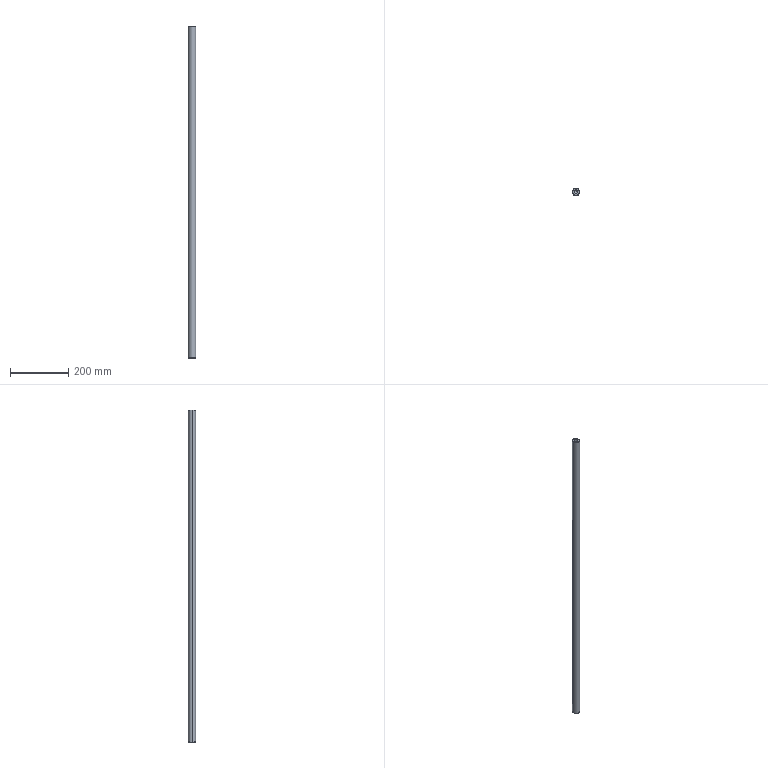Part | SolidWorks | features BaseBody 1 | 1 solid | 16 faces | box 25 x 25 x 1142 mm | volume 551182 mm3 | cone 8 | cylinder 6 | plane 2 | commonest cylinder face diameters 12 x4 25 x2
STEP:
#1=CARTESIAN_POINT('',(-11.5,0.,-571.));
#2=VERTEX_POINT('',#1);
#3=CARTESIAN_POINT('',(-12.5,0.,-570.));
#4=VERTEX_POINT('',#3);
#5=CARTESIAN_POINT('',(-12.5,0.,-570.));
#6=DIRECTION('',(-0.7071,0.,0.7071));
#7=VECTOR('',#6,1000.);
#8=LINE('',#5,#7);
#9=EDGE_CURVE('',#2,#4,#8,.T.);
#10=ORIENTED_EDGE('',*,*,#9,.F.);
#11=CARTESIAN_POINT('',(11.5,0.,-571.));
#12=VERTEX_POINT('',#11);
#13=CARTESIAN_POINT('',(0.,0.,-571.));
#14=DIRECTION('',(0.,0.,-1.));
#15=DIRECTION('',(1.,0.,0.));
#16=AXIS2_PLACEMENT_3D('',#13,#14,#15);
#17=CIRCLE('',#16,11.5);
#18=EDGE_CURVE('',#12,#2,#17,.T.);
#19=ORIENTED_EDGE('',*,*,#18,.F.);
#20=CARTESIAN_POINT('',(12.5,0.,-570.));
#21=VERTEX_POINT('',#20);
#22=CARTESIAN_POINT('',(12.5,0.,-570.));
#23=DIRECTION('',(0.7071,0.,0.7071));
#24=VECTOR('',#23,1000.);
#25=LINE('',#22,#24);
#26=EDGE_CURVE('',#12,#21,#25,.T.);
#27=ORIENTED_EDGE('',*,*,#26,.T.);
#28=CARTESIAN_POINT('',(0.,0.,-570.));
#29=DIRECTION('',(0.,0.,1.));
#30=DIRECTION('',(1.,0.,0.));
#31=AXIS2_PLACEMENT_3D('',#28,#29,#30);
#32=CIRCLE('',#31,12.5);
#33=EDGE_CURVE('',#4,#21,#32,.T.);
#34=ORIENTED_EDGE('',*,*,#33,.F.);
#35=EDGE_LOOP('',(#10,#19,#27,#34));
#36=FACE_OUTER_BOUND('',#35,.T.);
#37=CARTESIAN_POINT('',(0.,0.,-570.));
#38=DIRECTION('',(0.,0.,1.));
#39=DIRECTION('',(1.,0.,0.));
#40=AXIS2_PLACEMENT_3D('',#37,#38,#39);
#41=CONICAL_SURFACE('',#40,12.5,0.7854);
#42=ADVANCED_FACE('',(#36),#41,.T.);
#43=CARTESIAN_POINT('',(11.5,0.,571.));
#44=VERTEX_POINT('',#43);
#45=CARTESIAN_POINT('',(12.5,0.,570.));
#46=VERTEX_POINT('',#45);
#47=CARTESIAN_POINT('',(11.5,0.,571.));
#48=DIRECTION('',(0.7071,0.,-0.7071));
#49=VECTOR('',#48,1000.);
#50=LINE('',#47,#49);
#51=EDGE_CURVE('',#44,#46,#50,.T.);
#52=ORIENTED_EDGE('',*,*,#51,.F.);
#53=CARTESIAN_POINT('',(-11.5,0.,571.));
#54=VERTEX_POINT('',#53);
#55=CARTESIAN_POINT('',(0.,0.,571.));
#56=DIRECTION('',(0.,0.,1.));
#57=DIRECTION('',(1.,0.,0.));
#58=AXIS2_PLACEMENT_3D('',#55,#56,#57);
#59=CIRCLE('',#58,11.5);
#60=EDGE_CURVE('',#54,#44,#59,.T.);
#61=ORIENTED_EDGE('',*,*,#60,.F.);
#62=CARTESIAN_POINT('',(-12.5,0.,570.));
#63=VERTEX_POINT('',#62);
#64=CARTESIAN_POINT('',(-11.5,0.,571.));
#65=DIRECTION('',(-0.7071,0.,-0.7071));
#66=VECTOR('',#65,1000.);
#67=LINE('',#64,#66);
#68=EDGE_CURVE('',#54,#63,#67,.T.);
#69=ORIENTED_EDGE('',*,*,#68,.T.);
#70=CARTESIAN_POINT('',(0.,0.,570.));
#71=DIRECTION('',(0.,0.,-1.));
#72=DIRECTION('',(1.,0.,0.));
#73=AXIS2_PLACEMENT_3D('',#70,#71,#72);
#74=CIRCLE('',#73,12.5);
#75=EDGE_CURVE('',#46,#63,#74,.T.);
#76=ORIENTED_EDGE('',*,*,#75,.F.);
#77=EDGE_LOOP('',(#52,#61,#69,#76));
#78=FACE_OUTER_BOUND('',#77,.T.);
#79=CARTESIAN_POINT('',(0.,0.,571.));
#80=DIRECTION('',(0.,0.,-1.));
#81=DIRECTION('',(-1.,0.,0.));
#82=AXIS2_PLACEMENT_3D('',#79,#80,#81);
#83=CONICAL_SURFACE('',#82,11.5,0.7854);
#84=ADVANCED_FACE('',(#78),#83,.T.);
#85=CARTESIAN_POINT('',(6.,0.,-531.));
#86=VERTEX_POINT('',#85);
#87=CARTESIAN_POINT('',(6.,0.,-571.));
#88=VERTEX_POINT('',#87);
#89=CARTESIAN_POINT('',(6.,0.,-571.));
#90=DIRECTION('',(0.,0.,-1.));
#91=VECTOR('',#90,1000.);
#92=LINE('',#89,#91);
#93=EDGE_CURVE('',#86,#88,#92,.T.);
#94=ORIENTED_EDGE('',*,*,#93,.F.);
#95=CARTESIAN_POINT('',(-6.,0.,-531.));
#96=VERTEX_POINT('',#95);
#97=CARTESIAN_POINT('',(0.,0.,-531.));
#98=DIRECTION('',(0.,0.,-1.));
#99=DIRECTION('',(-1.,0.,0.));
#100=AXIS2_PLACEMENT_3D('',#97,#98,#99);
#101=CIRCLE('',#100,6.);
#102=EDGE_CURVE('',#96,#86,#101,.T.);
#103=ORIENTED_EDGE('',*,*,#102,.F.);
#104=CARTESIAN_POINT('',(-6.,0.,-571.));
#105=VERTEX_POINT('',#104);
#106=CARTESIAN_POINT('',(-6.,0.,-571.));
#107=DIRECTION('',(0.,0.,-1.));
#108=VECTOR('',#107,1000.);
#109=LINE('',#106,#108);
#110=EDGE_CURVE('',#96,#105,#109,.T.);
#111=ORIENTED_EDGE('',*,*,#110,.T.);
#112=CARTESIAN_POINT('',(0.,0.,-571.));
#113=DIRECTION('',(0.,0.,-1.));
#114=DIRECTION('',(-1.,0.,0.));
#115=AXIS2_PLACEMENT_3D('',#112,#113,#114);
#116=CIRCLE('',#115,6.);
#117=EDGE_CURVE('',#105,#88,#116,.T.);
#118=ORIENTED_EDGE('',*,*,#117,.T.);
#119=EDGE_LOOP('',(#94,#103,#111,#118));
#120=FACE_OUTER_BOUND('',#119,.T.);
#121=CARTESIAN_POINT('',(0.,0.,-571.));
#122=DIRECTION('',(0.,0.,-1.));
#123=DIRECTION('',(-1.,0.,0.));
#124=AXIS2_PLACEMENT_3D('',#121,#122,#123);
#125=CYLINDRICAL_SURFACE('',#124,6.);
#126=ADVANCED_FACE('',(#120),#125,.F.);
#127=CARTESIAN_POINT('',(0.,0.,-527.395));
#128=VERTEX_POINT('',#127);
#129=CARTESIAN_POINT('',(6.,0.,-531.));
#130=DIRECTION('',(0.8572,0.,-0.515));
#131=VECTOR('',#130,1000.);
#132=LINE('',#129,#131);
#133=EDGE_CURVE('',#128,#86,#132,.T.);
#134=ORIENTED_EDGE('',*,*,#133,.F.);
#135=CARTESIAN_POINT('',(-6.,0.,-531.));
#136=DIRECTION('',(-0.8572,0.,-0.515));
#137=VECTOR('',#136,1000.);
#138=LINE('',#135,#137);
#139=EDGE_CURVE('',#128,#96,#138,.T.);
#140=ORIENTED_EDGE('',*,*,#139,.T.);
#141=ORIENTED_EDGE('',*,*,#102,.T.);
#142=EDGE_LOOP('',(#134,#140,#141));
#143=FACE_OUTER_BOUND('',#142,.T.);
#144=CARTESIAN_POINT('',(0.,0.,-531.));
#145=DIRECTION('',(0.,0.,-1.));
#146=DIRECTION('',(-1.,0.,0.));
#147=AXIS2_PLACEMENT_3D('',#144,#145,#146);
#148=CONICAL_SURFACE('',#147,6.,1.03);
#149=ADVANCED_FACE('',(#143),#148,.F.);
#150=CARTESIAN_POINT('',(-6.,0.,531.));
#151=VERTEX_POINT('',#150);
#152=CARTESIAN_POINT('',(-6.,0.,571.));
#153=VERTEX_POINT('',#152);
#154=CARTESIAN_POINT('',(-6.,0.,571.));
#155=DIRECTION('',(0.,0.,1.));
#156=VECTOR('',#155,1000.);
#157=LINE('',#154,#156);
#158=EDGE_CURVE('',#151,#153,#157,.T.);
#159=ORIENTED_EDGE('',*,*,#158,.F.);
#160=CARTESIAN_POINT('',(6.,0.,531.));
#161=VERTEX_POINT('',#160);
#162=CARTESIAN_POINT('',(0.,0.,531.));
#163=DIRECTION('',(0.,0.,1.));
#164=DIRECTION('',(1.,0.,0.));
#165=AXIS2_PLACEMENT_3D('',#162,#163,#164);
#166=CIRCLE('',#165,6.);
#167=EDGE_CURVE('',#161,#151,#166,.T.);
#168=ORIENTED_EDGE('',*,*,#167,.F.);
#169=CARTESIAN_POINT('',(6.,0.,571.));
#170=VERTEX_POINT('',#169);
#171=CARTESIAN_POINT('',(6.,0.,571.));
#172=DIRECTION('',(0.,0.,1.));
#173=VECTOR('',#172,1000.);
#174=LINE('',#171,#173);
#175=EDGE_CURVE('',#161,#170,#174,.T.);
#176=ORIENTED_EDGE('',*,*,#175,.T.);
#177=CARTESIAN_POINT('',(0.,0.,571.));
#178=DIRECTION('',(0.,0.,1.));
#179=DIRECTION('',(1.,0.,0.));
#180=AXIS2_PLACEMENT_3D('',#177,#178,#179);
#181=CIRCLE('',#180,6.);
#182=EDGE_CURVE('',#170,#153,#181,.T.);
#183=ORIENTED_EDGE('',*,*,#182,.T.);
#184=EDGE_LOOP('',(#159,#168,#176,#183));
#185=FACE_OUTER_BOUND('',#184,.T.);
#186=CARTESIAN_POINT('',(0.,0.,571.));
#187=DIRECTION('',(0.,0.,1.));
#188=DIRECTION('',(1.,0.,0.));
#189=AXIS2_PLACEMENT_3D('',#186,#187,#188);
#190=CYLINDRICAL_SURFACE('',#189,6.);
#191=ADVANCED_FACE('',(#185),#190,.F.);
#192=CARTESIAN_POINT('',(0.,0.,527.395));
#193=VERTEX_POINT('',#192);
#194=CARTESIAN_POINT('',(-6.,0.,531.));
#195=DIRECTION('',(-0.8572,0.,0.515));
#196=VECTOR('',#195,1000.);
#197=LINE('',#194,#196);
#198=EDGE_CURVE('',#193,#151,#197,.T.);
#199=ORIENTED_EDGE('',*,*,#198,.F.);
#200=CARTESIAN_POINT('',(6.,0.,531.));
#201=DIRECTION('',(0.8572,0.,0.515));
#202=VECTOR('',#201,1000.);
#203=LINE('',#200,#202);
#204=EDGE_CURVE('',#193,#161,#203,.T.);
#205=ORIENTED_EDGE('',*,*,#204,.T.);
#206=ORIENTED_EDGE('',*,*,#167,.T.);
#207=EDGE_LOOP('',(#199,#205,#206));
#208=FACE_OUTER_BOUND('',#207,.T.);
#209=CARTESIAN_POINT('',(0.,0.,531.));
#210=DIRECTION('',(0.,0.,1.));
#211=DIRECTION('',(1.,0.,0.));
#212=AXIS2_PLACEMENT_3D('',#209,#210,#211);
#213=CONICAL_SURFACE('',#212,6.,1.03);
#214=ADVANCED_FACE('',(#208),#213,.F.);
#215=ORIENTED_EDGE('',*,*,#117,.F.);
#216=CARTESIAN_POINT('',(0.,0.,-571.));
#217=DIRECTION('',(0.,0.,-1.));
#218=DIRECTION('',(-1.,0.,0.));
#219=AXIS2_PLACEMENT_3D('',#216,#217,#218);
#220=CIRCLE('',#219,6.);
#221=EDGE_CURVE('',#88,#105,#220,.T.);
#222=ORIENTED_EDGE('',*,*,#221,.F.);
#223=EDGE_LOOP('',(#215,#222));
#224=FACE_BOUND('',#223,.T.);
#225=ORIENTED_EDGE('',*,*,#18,.T.);
#226=CARTESIAN_POINT('',(0.,0.,-571.));
#227=DIRECTION('',(0.,0.,-1.));
#228=DIRECTION('',(1.,0.,0.));
#229=AXIS2_PLACEMENT_3D('',#226,#227,#228);
#230=CIRCLE('',#229,11.5);
#231=EDGE_CURVE('',#2,#12,#230,.T.);
#232=ORIENTED_EDGE('',*,*,#231,.T.);
#233=EDGE_LOOP('',(#225,#232));
#234=FACE_OUTER_BOUND('',#233,.T.);
#235=CARTESIAN_POINT('',(0.,0.,-571.));
#236=DIRECTION('',(0.,0.,1.));
#237=DIRECTION('',(1.,0.,0.));
#238=AXIS2_PLACEMENT_3D('',#235,#236,#237);
#239=PLANE('',#238);
#240=ADVANCED_FACE('',(#224,#234),#239,.F.);
#241=ORIENTED_EDGE('',*,*,#182,.F.);
#242=CARTESIAN_POINT('',(0.,0.,571.));
#243=DIRECTION('',(0.,0.,1.));
#244=DIRECTION('',(1.,0.,0.));
#245=AXIS2_PLACEMENT_3D('',#242,#243,#244);
#246=CIRCLE('',#245,6.);
#247=EDGE_CURVE('',#153,#170,#246,.T.);
#248=ORIENTED_EDGE('',*,*,#247,.F.);
#249=EDGE_LOOP('',(#241,#248));
#250=FACE_BOUND('',#249,.T.);
#251=ORIENTED_EDGE('',*,*,#60,.T.);
#252=CARTESIAN_POINT('',(0.,0.,571.));
#253=DIRECTION('',(0.,0.,1.));
#254=DIRECTION('',(1.,0.,0.));
#255=AXIS2_PLACEMENT_3D('',#252,#253,#254);
#256=CIRCLE('',#255,11.5);
#257=EDGE_CURVE('',#44,#54,#256,.T.);
#258=ORIENTED_EDGE('',*,*,#257,.T.);
#259=EDGE_LOOP('',(#251,#258));
#260=FACE_OUTER_BOUND('',#259,.T.);
#261=CARTESIAN_POINT('',(0.,0.,571.));
#262=DIRECTION('',(0.,0.,1.));
#263=DIRECTION('',(1.,0.,0.));
#264=AXIS2_PLACEMENT_3D('',#261,#262,#263);
#265=PLANE('',#264);
#266=ADVANCED_FACE('',(#250,#260),#265,.T.);
#267=CARTESIAN_POINT('',(12.5,0.,571.));
#268=DIRECTION('',(0.,0.,-1.));
#269=VECTOR('',#268,1000.);
#270=LINE('',#267,#269);
#271=EDGE_CURVE('',#46,#21,#270,.T.);
#272=ORIENTED_EDGE('',*,*,#271,.F.);
#273=ORIENTED_EDGE('',*,*,#75,.T.);
#274=CARTESIAN_POINT('',(-12.5,0.,571.));
#275=DIRECTION('',(0.,0.,-1.));
#276=VECTOR('',#275,1000.);
#277=LINE('',#274,#276);
#278=EDGE_CURVE('',#63,#4,#277,.T.);
#279=ORIENTED_EDGE('',*,*,#278,.T.);
#280=ORIENTED_EDGE('',*,*,#33,.T.);
#281=EDGE_LOOP('',(#272,#273,#279,#280));
#282=FACE_OUTER_BOUND('',#281,.T.);
#283=CARTESIAN_POINT('',(0.,0.,571.));
#284=DIRECTION('',(0.,0.,-1.));
#285=DIRECTION('',(-1.,0.,0.));
#286=AXIS2_PLACEMENT_3D('',#283,#284,#285);
#287=CYLINDRICAL_SURFACE('',#286,12.5);
#288=ADVANCED_FACE('',(#282),#287,.T.);
#289=CARTESIAN_POINT('',(0.,0.,570.));
#290=DIRECTION('',(0.,0.,-1.));
#291=DIRECTION('',(1.,0.,0.));
#292=AXIS2_PLACEMENT_3D('',#289,#290,#291);
#293=CIRCLE('',#292,12.5);
#294=EDGE_CURVE('',#63,#46,#293,.T.);
#295=ORIENTED_EDGE('',*,*,#294,.T.);
#296=ORIENTED_EDGE('',*,*,#271,.T.);
#297=CARTESIAN_POINT('',(0.,0.,-570.));
#298=DIRECTION('',(0.,0.,1.));
#299=DIRECTION('',(1.,0.,0.));
#300=AXIS2_PLACEMENT_3D('',#297,#298,#299);
#301=CIRCLE('',#300,12.5);
#302=EDGE_CURVE('',#21,#4,#301,.T.);
#303=ORIENTED_EDGE('',*,*,#302,.T.);
#304=ORIENTED_EDGE('',*,*,#278,.F.);
#305=EDGE_LOOP('',(#295,#296,#303,#304));
#306=FACE_OUTER_BOUND('',#305,.T.);
#307=CARTESIAN_POINT('',(0.,0.,571.));
#308=DIRECTION('',(0.,0.,-1.));
#309=DIRECTION('',(-1.,0.,0.));
#310=AXIS2_PLACEMENT_3D('',#307,#308,#309);
#311=CYLINDRICAL_SURFACE('',#310,12.5);
#312=ADVANCED_FACE('',(#306),#311,.T.);
#313=ORIENTED_EDGE('',*,*,#204,.F.);
#314=ORIENTED_EDGE('',*,*,#198,.T.);
#315=CARTESIAN_POINT('',(0.,0.,531.));
#316=DIRECTION('',(0.,0.,1.));
#317=DIRECTION('',(1.,0.,0.));
#318=AXIS2_PLACEMENT_3D('',#315,#316,#317);
#319=CIRCLE('',#318,6.);
#320=EDGE_CURVE('',#151,#161,#319,.T.);
#321=ORIENTED_EDGE('',*,*,#320,.T.);
#322=EDGE_LOOP('',(#313,#314,#321));
#323=FACE_OUTER_BOUND('',#322,.T.);
#324=CARTESIAN_POINT('',(0.,0.,531.));
#325=DIRECTION('',(0.,0.,1.));
#326=DIRECTION('',(1.,0.,0.));
#327=AXIS2_PLACEMENT_3D('',#324,#325,#326);
#328=CONICAL_SURFACE('',#327,6.,1.03);
#329=ADVANCED_FACE('',(#323),#328,.F.);
#330=ORIENTED_EDGE('',*,*,#320,.F.);
#331=ORIENTED_EDGE('',*,*,#158,.T.);
#332=ORIENTED_EDGE('',*,*,#247,.T.);
#333=ORIENTED_EDGE('',*,*,#175,.F.);
#334=EDGE_LOOP('',(#330,#331,#332,#333));
#335=FACE_OUTER_BOUND('',#334,.T.);
#336=CARTESIAN_POINT('',(0.,0.,571.));
#337=DIRECTION('',(0.,0.,1.));
#338=DIRECTION('',(1.,0.,0.));
#339=AXIS2_PLACEMENT_3D('',#336,#337,#338);
#340=CYLINDRICAL_SURFACE('',#339,6.);
#341=ADVANCED_FACE('',(#335),#340,.F.);
#342=ORIENTED_EDGE('',*,*,#139,.F.);
#343=ORIENTED_EDGE('',*,*,#133,.T.);
#344=CARTESIAN_POINT('',(0.,0.,-531.));
#345=DIRECTION('',(0.,0.,-1.));
#346=DIRECTION('',(-1.,0.,0.));
#347=AXIS2_PLACEMENT_3D('',#344,#345,#346);
#348=CIRCLE('',#347,6.);
#349=EDGE_CURVE('',#86,#96,#348,.T.);
#350=ORIENTED_EDGE('',*,*,#349,.T.);
#351=EDGE_LOOP('',(#342,#343,#350));
#352=FACE_OUTER_BOUND('',#351,.T.);
#353=CARTESIAN_POINT('',(0.,0.,-531.));
#354=DIRECTION('',(0.,0.,-1.));
#355=DIRECTION('',(-1.,0.,0.));
#356=AXIS2_PLACEMENT_3D('',#353,#354,#355);
#357=CONICAL_SURFACE('',#356,6.,1.03);
#358=ADVANCED_FACE('',(#352),#357,.F.);
#359=ORIENTED_EDGE('',*,*,#349,.F.);
#360=ORIENTED_EDGE('',*,*,#93,.T.);
#361=ORIENTED_EDGE('',*,*,#221,.T.);
#362=ORIENTED_EDGE('',*,*,#110,.F.);
#363=EDGE_LOOP('',(#359,#360,#361,#362));
#364=FACE_OUTER_BOUND('',#363,.T.);
#365=CARTESIAN_POINT('',(0.,0.,-571.));
#366=DIRECTION('',(0.,0.,-1.));
#367=DIRECTION('',(-1.,0.,0.));
#368=AXIS2_PLACEMENT_3D('',#365,#366,#367);
#369=CYLINDRICAL_SURFACE('',#368,6.);
#370=ADVANCED_FACE('',(#364),#369,.F.);
#371=ORIENTED_EDGE('',*,*,#257,.F.);
#372=ORIENTED_EDGE('',*,*,#51,.T.);
#373=ORIENTED_EDGE('',*,*,#294,.F.);
#374=ORIENTED_EDGE('',*,*,#68,.F.);
#375=EDGE_LOOP('',(#371,#372,#373,#374));
#376=FACE_OUTER_BOUND('',#375,.T.);
#377=CARTESIAN_POINT('',(0.,0.,571.));
#378=DIRECTION('',(0.,0.,-1.));
#379=DIRECTION('',(-1.,0.,0.));
#380=AXIS2_PLACEMENT_3D('',#377,#378,#379);
#381=CONICAL_SURFACE('',#380,11.5,0.7854);
#382=ADVANCED_FACE('',(#376),#381,.T.);
#383=ORIENTED_EDGE('',*,*,#231,.F.);
#384=ORIENTED_EDGE('',*,*,#9,.T.);
#385=ORIENTED_EDGE('',*,*,#302,.F.);
#386=ORIENTED_EDGE('',*,*,#26,.F.);
#387=EDGE_LOOP('',(#383,#384,#385,#386));
#388=FACE_OUTER_BOUND('',#387,.T.);
#389=CARTESIAN_POINT('',(0.,0.,-570.));
#390=DIRECTION('',(0.,0.,1.));
#391=DIRECTION('',(1.,0.,0.));
#392=AXIS2_PLACEMENT_3D('',#389,#390,#391);
#393=CONICAL_SURFACE('',#392,12.5,0.7854);
#394=ADVANCED_FACE('',(#388),#393,.T.);
#395=CLOSED_SHELL('',(#42,#84,#126,#149,#191,#214,#240,#266,#288,#312,#329,#341,#358,#370,#382,#394));
#396=MANIFOLD_SOLID_BREP('',#395);
#397=CARTESIAN_POINT('',(0.,0.,0.));
#398=DIRECTION('',(0.,0.,1.));
#399=DIRECTION('',(1.,0.,0.));
#400=AXIS2_PLACEMENT_3D('',#397,#398,#399);
#401=(LENGTH_UNIT()NAMED_UNIT(*)SI_UNIT(.MILLI.,.METRE.));
#402=UNCERTAINTY_MEASURE_WITH_UNIT(LENGTH_MEASURE(0.00001),#401,'','');
#403=(NAMED_UNIT(*)PLANE_ANGLE_UNIT()SI_UNIT($,.RADIAN.));
#404=(NAMED_UNIT(*)SI_UNIT($,.STERADIAN.)SOLID_ANGLE_UNIT());
#405=(GEOMETRIC_REPRESENTATION_CONTEXT(3)GLOBAL_UNCERTAINTY_ASSIGNED_CONTEXT((#402))GLOBAL_UNIT_ASSIGNED_CONTEXT((#401,#403,#404))REPRESENTATION_CONTEXT('',''));
#406=ADVANCED_BREP_SHAPE_REPRESENTATION('',(#396,#400),#405);